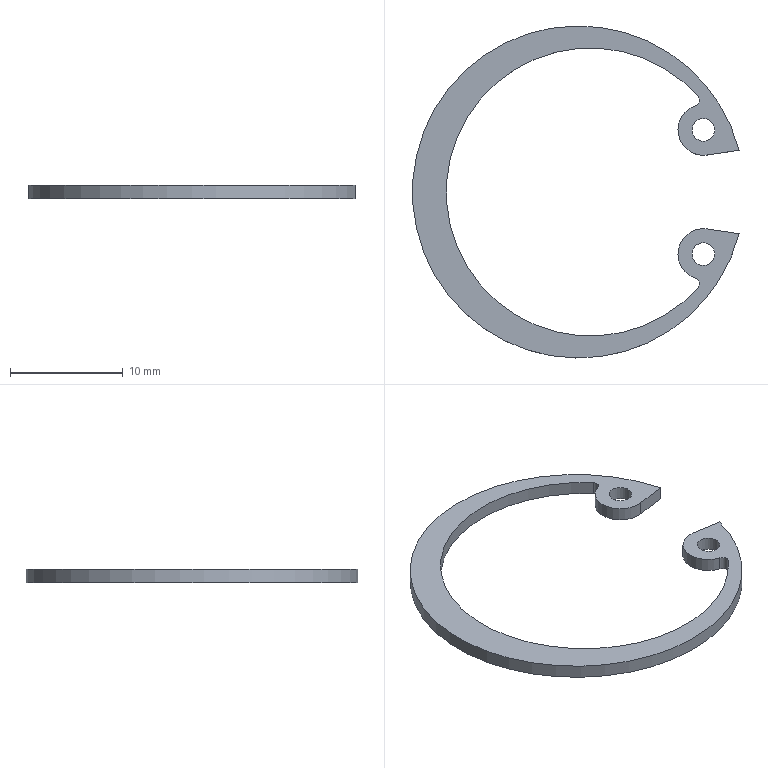Part | NX | features Retaining Ring C In-1_5003_005_BGRB6902ZZ-25 2 | 1 solid | 12 faces | box 28.927 x 29.4 x 1.2 mm | volume 220.032 mm3 | cylinder 8 | plane 4 | commonest cylinder face diameters 1 x2 2 x2 4.498 x2 25.5 x1 29.4 x1
STEP:
#1=CARTESIAN_POINT('',(169.581,-317.5,-237.85));
#2=VERTEX_POINT('',#1);
#3=CARTESIAN_POINT('',(169.581,-316.5,-237.85));
#4=DIRECTION('',(0.,0.,-1.));
#5=DIRECTION('',(0.,-1.,0.));
#6=AXIS2_PLACEMENT_3D('',#3,#4,#5);
#7=CIRCLE('',#6,1.);
#8=EDGE_CURVE('',#2,#2,#7,.T.);
#9=ORIENTED_EDGE('',*,*,#8,.F.);
#10=EDGE_LOOP('',(#9));
#11=FACE_BOUND('',#10,.T.);
#12=CARTESIAN_POINT('',(169.914,-318.724,-237.85));
#13=VERTEX_POINT('',#12);
#14=CARTESIAN_POINT('',(168.899,-314.357,-237.85));
#15=VERTEX_POINT('',#14);
#16=CARTESIAN_POINT('',(169.581,-316.5,-237.85));
#17=DIRECTION('',(0.,0.,-1.));
#18=DIRECTION('',(0.,-1.,0.));
#19=AXIS2_PLACEMENT_3D('',#16,#17,#18);
#20=CIRCLE('',#19,2.249);
#21=EDGE_CURVE('',#13,#15,#20,.T.);
#22=ORIENTED_EDGE('',*,*,#21,.T.);
#23=CARTESIAN_POINT('',(169.122,-313.549,-237.85));
#24=VERTEX_POINT('',#23);
#25=CARTESIAN_POINT('',(168.748,-313.881,-237.85));
#26=DIRECTION('',(0.,0.,1.));
#27=DIRECTION('',(0.,-1.,0.));
#28=AXIS2_PLACEMENT_3D('',#25,#26,#27);
#29=CIRCLE('',#28,0.5);
#30=EDGE_CURVE('',#15,#24,#29,.T.);
#31=ORIENTED_EDGE('',*,*,#30,.T.);
#32=CARTESIAN_POINT('',(169.122,-330.451,-237.85));
#33=VERTEX_POINT('',#32);
#34=CARTESIAN_POINT('',(159.575,-322.,-237.85));
#35=DIRECTION('',(0.,0.,1.));
#36=DIRECTION('',(0.,-1.,0.));
#37=AXIS2_PLACEMENT_3D('',#34,#35,#36);
#38=CIRCLE('',#37,12.75);
#39=EDGE_CURVE('',#24,#33,#38,.T.);
#40=ORIENTED_EDGE('',*,*,#39,.T.);
#41=CARTESIAN_POINT('',(168.899,-329.643,-237.85));
#42=VERTEX_POINT('',#41);
#43=CARTESIAN_POINT('',(168.748,-330.119,-237.85));
#44=DIRECTION('',(0.,0.,1.));
#45=DIRECTION('',(0.,1.,0.));
#46=AXIS2_PLACEMENT_3D('',#43,#44,#45);
#47=CIRCLE('',#46,0.5);
#48=EDGE_CURVE('',#33,#42,#47,.T.);
#49=ORIENTED_EDGE('',*,*,#48,.T.);
#50=CARTESIAN_POINT('',(169.914,-325.276,-237.85));
#51=VERTEX_POINT('',#50);
#52=CARTESIAN_POINT('',(169.581,-327.5,-237.85));
#53=DIRECTION('',(0.,0.,-1.));
#54=DIRECTION('',(0.,-1.,0.));
#55=AXIS2_PLACEMENT_3D('',#52,#53,#54);
#56=CIRCLE('',#55,2.249);
#57=EDGE_CURVE('',#42,#51,#56,.T.);
#58=ORIENTED_EDGE('',*,*,#57,.T.);
#59=CARTESIAN_POINT('',(172.752,-325.7,-237.85));
#60=VERTEX_POINT('',#59);
#61=CARTESIAN_POINT('',(169.914,-325.276,-237.85));
#62=DIRECTION('',(0.989,-0.1478,0.));
#63=VECTOR('',#62,1000.);
#64=LINE('',#61,#63);
#65=EDGE_CURVE('',#51,#60,#64,.T.);
#66=ORIENTED_EDGE('',*,*,#65,.T.);
#67=CARTESIAN_POINT('',(172.752,-318.3,-237.85));
#68=VERTEX_POINT('',#67);
#69=CARTESIAN_POINT('',(158.525,-322.,-237.85));
#70=DIRECTION('',(0.,0.,-1.));
#71=DIRECTION('',(0.,-1.,0.));
#72=AXIS2_PLACEMENT_3D('',#69,#70,#71);
#73=CIRCLE('',#72,14.7);
#74=EDGE_CURVE('',#60,#68,#73,.T.);
#75=ORIENTED_EDGE('',*,*,#74,.T.);
#76=CARTESIAN_POINT('',(169.914,-318.724,-237.85));
#77=DIRECTION('',(-0.989,-0.1478,0.));
#78=VECTOR('',#77,1000.);
#79=LINE('',#76,#78);
#80=EDGE_CURVE('',#68,#13,#79,.T.);
#81=ORIENTED_EDGE('',*,*,#80,.T.);
#82=EDGE_LOOP('',(#22,#31,#40,#49,#58,#66,#75,#81));
#83=FACE_BOUND('',#82,.T.);
#84=CARTESIAN_POINT('',(169.581,-328.5,-237.85));
#85=VERTEX_POINT('',#84);
#86=CARTESIAN_POINT('',(169.581,-327.5,-237.85));
#87=DIRECTION('',(0.,0.,-1.));
#88=DIRECTION('',(0.,-1.,0.));
#89=AXIS2_PLACEMENT_3D('',#86,#87,#88);
#90=CIRCLE('',#89,1.);
#91=EDGE_CURVE('',#85,#85,#90,.T.);
#92=ORIENTED_EDGE('',*,*,#91,.F.);
#93=EDGE_LOOP('',(#92));
#94=FACE_BOUND('',#93,.T.);
#95=CARTESIAN_POINT('',(169.581,-316.5,-237.85));
#96=DIRECTION('',(0.,0.,-1.));
#97=DIRECTION('',(0.,-1.,0.));
#98=AXIS2_PLACEMENT_3D('',#95,#96,#97);
#99=PLANE('',#98);
#100=ADVANCED_FACE('',(#11,#83,#94),#99,.T.);
#101=CARTESIAN_POINT('',(169.581,-317.5,-236.65));
#102=VERTEX_POINT('',#101);
#103=CARTESIAN_POINT('',(169.581,-316.5,-236.65));
#104=DIRECTION('',(0.,0.,-1.));
#105=DIRECTION('',(0.,-1.,0.));
#106=AXIS2_PLACEMENT_3D('',#103,#104,#105);
#107=CIRCLE('',#106,1.);
#108=EDGE_CURVE('',#102,#102,#107,.T.);
#109=ORIENTED_EDGE('',*,*,#108,.T.);
#110=EDGE_LOOP('',(#109));
#111=FACE_BOUND('',#110,.T.);
#112=CARTESIAN_POINT('',(169.914,-318.724,-236.65));
#113=VERTEX_POINT('',#112);
#114=CARTESIAN_POINT('',(168.899,-314.357,-236.65));
#115=VERTEX_POINT('',#114);
#116=CARTESIAN_POINT('',(169.581,-316.5,-236.65));
#117=DIRECTION('',(0.,0.,-1.));
#118=DIRECTION('',(0.,-1.,0.));
#119=AXIS2_PLACEMENT_3D('',#116,#117,#118);
#120=CIRCLE('',#119,2.249);
#121=EDGE_CURVE('',#113,#115,#120,.T.);
#122=ORIENTED_EDGE('',*,*,#121,.F.);
#123=CARTESIAN_POINT('',(172.752,-318.3,-236.65));
#124=VERTEX_POINT('',#123);
#125=CARTESIAN_POINT('',(169.914,-318.724,-236.65));
#126=DIRECTION('',(-0.989,-0.1478,0.));
#127=VECTOR('',#126,1000.);
#128=LINE('',#125,#127);
#129=EDGE_CURVE('',#124,#113,#128,.T.);
#130=ORIENTED_EDGE('',*,*,#129,.F.);
#131=CARTESIAN_POINT('',(172.752,-325.7,-236.65));
#132=VERTEX_POINT('',#131);
#133=CARTESIAN_POINT('',(158.525,-322.,-236.65));
#134=DIRECTION('',(0.,0.,-1.));
#135=DIRECTION('',(0.,-1.,0.));
#136=AXIS2_PLACEMENT_3D('',#133,#134,#135);
#137=CIRCLE('',#136,14.7);
#138=EDGE_CURVE('',#132,#124,#137,.T.);
#139=ORIENTED_EDGE('',*,*,#138,.F.);
#140=CARTESIAN_POINT('',(169.914,-325.276,-236.65));
#141=VERTEX_POINT('',#140);
#142=CARTESIAN_POINT('',(169.914,-325.276,-236.65));
#143=DIRECTION('',(0.989,-0.1478,0.));
#144=VECTOR('',#143,1000.);
#145=LINE('',#142,#144);
#146=EDGE_CURVE('',#141,#132,#145,.T.);
#147=ORIENTED_EDGE('',*,*,#146,.F.);
#148=CARTESIAN_POINT('',(168.899,-329.643,-236.65));
#149=VERTEX_POINT('',#148);
#150=CARTESIAN_POINT('',(169.581,-327.5,-236.65));
#151=DIRECTION('',(0.,0.,-1.));
#152=DIRECTION('',(0.,-1.,0.));
#153=AXIS2_PLACEMENT_3D('',#150,#151,#152);
#154=CIRCLE('',#153,2.249);
#155=EDGE_CURVE('',#149,#141,#154,.T.);
#156=ORIENTED_EDGE('',*,*,#155,.F.);
#157=CARTESIAN_POINT('',(169.122,-330.451,-236.65));
#158=VERTEX_POINT('',#157);
#159=CARTESIAN_POINT('',(168.748,-330.119,-236.65));
#160=DIRECTION('',(0.,0.,1.));
#161=DIRECTION('',(0.,1.,0.));
#162=AXIS2_PLACEMENT_3D('',#159,#160,#161);
#163=CIRCLE('',#162,0.5);
#164=EDGE_CURVE('',#158,#149,#163,.T.);
#165=ORIENTED_EDGE('',*,*,#164,.F.);
#166=CARTESIAN_POINT('',(169.122,-313.549,-236.65));
#167=VERTEX_POINT('',#166);
#168=CARTESIAN_POINT('',(159.575,-322.,-236.65));
#169=DIRECTION('',(0.,0.,1.));
#170=DIRECTION('',(0.,-1.,0.));
#171=AXIS2_PLACEMENT_3D('',#168,#169,#170);
#172=CIRCLE('',#171,12.75);
#173=EDGE_CURVE('',#167,#158,#172,.T.);
#174=ORIENTED_EDGE('',*,*,#173,.F.);
#175=CARTESIAN_POINT('',(168.748,-313.881,-236.65));
#176=DIRECTION('',(0.,0.,1.));
#177=DIRECTION('',(0.,-1.,0.));
#178=AXIS2_PLACEMENT_3D('',#175,#176,#177);
#179=CIRCLE('',#178,0.5);
#180=EDGE_CURVE('',#115,#167,#179,.T.);
#181=ORIENTED_EDGE('',*,*,#180,.F.);
#182=EDGE_LOOP('',(#122,#130,#139,#147,#156,#165,#174,#181));
#183=FACE_BOUND('',#182,.T.);
#184=CARTESIAN_POINT('',(169.581,-328.5,-236.65));
#185=VERTEX_POINT('',#184);
#186=CARTESIAN_POINT('',(169.581,-327.5,-236.65));
#187=DIRECTION('',(0.,0.,-1.));
#188=DIRECTION('',(0.,-1.,0.));
#189=AXIS2_PLACEMENT_3D('',#186,#187,#188);
#190=CIRCLE('',#189,1.);
#191=EDGE_CURVE('',#185,#185,#190,.T.);
#192=ORIENTED_EDGE('',*,*,#191,.T.);
#193=EDGE_LOOP('',(#192));
#194=FACE_BOUND('',#193,.T.);
#195=CARTESIAN_POINT('',(169.581,-316.5,-236.65));
#196=DIRECTION('',(0.,0.,-1.));
#197=DIRECTION('',(0.,-1.,0.));
#198=AXIS2_PLACEMENT_3D('',#195,#196,#197);
#199=PLANE('',#198);
#200=ADVANCED_FACE('',(#111,#183,#194),#199,.F.);
#201=ORIENTED_EDGE('',*,*,#121,.T.);
#202=CARTESIAN_POINT('',(168.899,-314.357,-237.85));
#203=DIRECTION('',(0.,0.,1.));
#204=VECTOR('',#203,1000.);
#205=LINE('',#202,#204);
#206=EDGE_CURVE('',#15,#115,#205,.T.);
#207=ORIENTED_EDGE('',*,*,#206,.F.);
#208=ORIENTED_EDGE('',*,*,#21,.F.);
#209=CARTESIAN_POINT('',(169.914,-318.724,-237.85));
#210=DIRECTION('',(0.,0.,1.));
#211=VECTOR('',#210,1000.);
#212=LINE('',#209,#211);
#213=EDGE_CURVE('',#13,#113,#212,.T.);
#214=ORIENTED_EDGE('',*,*,#213,.T.);
#215=EDGE_LOOP('',(#201,#207,#208,#214));
#216=FACE_BOUND('',#215,.T.);
#217=CARTESIAN_POINT('',(169.581,-316.5,-237.85));
#218=DIRECTION('',(0.,0.,1.));
#219=DIRECTION('',(0.,1.,0.));
#220=AXIS2_PLACEMENT_3D('',#217,#218,#219);
#221=CYLINDRICAL_SURFACE('',#220,2.249);
#222=ADVANCED_FACE('',(#216),#221,.T.);
#223=ORIENTED_EDGE('',*,*,#180,.T.);
#224=CARTESIAN_POINT('',(169.122,-313.549,-237.85));
#225=DIRECTION('',(0.,0.,1.));
#226=VECTOR('',#225,1000.);
#227=LINE('',#224,#226);
#228=EDGE_CURVE('',#24,#167,#227,.T.);
#229=ORIENTED_EDGE('',*,*,#228,.F.);
#230=ORIENTED_EDGE('',*,*,#30,.F.);
#231=ORIENTED_EDGE('',*,*,#206,.T.);
#232=EDGE_LOOP('',(#223,#229,#230,#231));
#233=FACE_BOUND('',#232,.T.);
#234=CARTESIAN_POINT('',(168.748,-313.881,-237.85));
#235=DIRECTION('',(0.,0.,1.));
#236=DIRECTION('',(0.,1.,0.));
#237=AXIS2_PLACEMENT_3D('',#234,#235,#236);
#238=CYLINDRICAL_SURFACE('',#237,0.5);
#239=ADVANCED_FACE('',(#233),#238,.F.);
#240=ORIENTED_EDGE('',*,*,#173,.T.);
#241=CARTESIAN_POINT('',(169.122,-330.451,-237.85));
#242=DIRECTION('',(0.,0.,1.));
#243=VECTOR('',#242,1000.);
#244=LINE('',#241,#243);
#245=EDGE_CURVE('',#33,#158,#244,.T.);
#246=ORIENTED_EDGE('',*,*,#245,.F.);
#247=ORIENTED_EDGE('',*,*,#39,.F.);
#248=ORIENTED_EDGE('',*,*,#228,.T.);
#249=EDGE_LOOP('',(#240,#246,#247,#248));
#250=FACE_BOUND('',#249,.T.);
#251=CARTESIAN_POINT('',(159.575,-322.,-237.85));
#252=DIRECTION('',(0.,0.,1.));
#253=DIRECTION('',(0.,1.,0.));
#254=AXIS2_PLACEMENT_3D('',#251,#252,#253);
#255=CYLINDRICAL_SURFACE('',#254,12.75);
#256=ADVANCED_FACE('',(#250),#255,.F.);
#257=ORIENTED_EDGE('',*,*,#164,.T.);
#258=CARTESIAN_POINT('',(168.899,-329.643,-237.85));
#259=DIRECTION('',(0.,0.,1.));
#260=VECTOR('',#259,1000.);
#261=LINE('',#258,#260);
#262=EDGE_CURVE('',#42,#149,#261,.T.);
#263=ORIENTED_EDGE('',*,*,#262,.F.);
#264=ORIENTED_EDGE('',*,*,#48,.F.);
#265=ORIENTED_EDGE('',*,*,#245,.T.);
#266=EDGE_LOOP('',(#257,#263,#264,#265));
#267=FACE_BOUND('',#266,.T.);
#268=CARTESIAN_POINT('',(168.748,-330.119,-237.85));
#269=DIRECTION('',(0.,0.,1.));
#270=DIRECTION('',(0.,1.,0.));
#271=AXIS2_PLACEMENT_3D('',#268,#269,#270);
#272=CYLINDRICAL_SURFACE('',#271,0.5);
#273=ADVANCED_FACE('',(#267),#272,.F.);
#274=ORIENTED_EDGE('',*,*,#155,.T.);
#275=CARTESIAN_POINT('',(169.914,-325.276,-237.85));
#276=DIRECTION('',(0.,0.,1.));
#277=VECTOR('',#276,1000.);
#278=LINE('',#275,#277);
#279=EDGE_CURVE('',#51,#141,#278,.T.);
#280=ORIENTED_EDGE('',*,*,#279,.F.);
#281=ORIENTED_EDGE('',*,*,#57,.F.);
#282=ORIENTED_EDGE('',*,*,#262,.T.);
#283=EDGE_LOOP('',(#274,#280,#281,#282));
#284=FACE_BOUND('',#283,.T.);
#285=CARTESIAN_POINT('',(169.581,-327.5,-237.85));
#286=DIRECTION('',(0.,0.,1.));
#287=DIRECTION('',(0.,1.,0.));
#288=AXIS2_PLACEMENT_3D('',#285,#286,#287);
#289=CYLINDRICAL_SURFACE('',#288,2.249);
#290=ADVANCED_FACE('',(#284),#289,.T.);
#291=ORIENTED_EDGE('',*,*,#146,.T.);
#292=CARTESIAN_POINT('',(172.752,-325.7,-237.85));
#293=DIRECTION('',(0.,0.,1.));
#294=VECTOR('',#293,1000.);
#295=LINE('',#292,#294);
#296=EDGE_CURVE('',#60,#132,#295,.T.);
#297=ORIENTED_EDGE('',*,*,#296,.F.);
#298=ORIENTED_EDGE('',*,*,#65,.F.);
#299=ORIENTED_EDGE('',*,*,#279,.T.);
#300=EDGE_LOOP('',(#291,#297,#298,#299));
#301=FACE_BOUND('',#300,.T.);
#302=CARTESIAN_POINT('',(169.914,-325.276,-237.85));
#303=DIRECTION('',(-0.1478,-0.989,0.));
#304=DIRECTION('',(-0.989,0.1478,0.));
#305=AXIS2_PLACEMENT_3D('',#302,#303,#304);
#306=PLANE('',#305);
#307=ADVANCED_FACE('',(#301),#306,.F.);
#308=ORIENTED_EDGE('',*,*,#138,.T.);
#309=CARTESIAN_POINT('',(172.752,-318.3,-237.85));
#310=DIRECTION('',(0.,0.,1.));
#311=VECTOR('',#310,1000.);
#312=LINE('',#309,#311);
#313=EDGE_CURVE('',#68,#124,#312,.T.);
#314=ORIENTED_EDGE('',*,*,#313,.F.);
#315=ORIENTED_EDGE('',*,*,#74,.F.);
#316=ORIENTED_EDGE('',*,*,#296,.T.);
#317=EDGE_LOOP('',(#308,#314,#315,#316));
#318=FACE_BOUND('',#317,.T.);
#319=CARTESIAN_POINT('',(158.525,-322.,-237.85));
#320=DIRECTION('',(0.,0.,1.));
#321=DIRECTION('',(0.,1.,0.));
#322=AXIS2_PLACEMENT_3D('',#319,#320,#321);
#323=CYLINDRICAL_SURFACE('',#322,14.7);
#324=ADVANCED_FACE('',(#318),#323,.T.);
#325=ORIENTED_EDGE('',*,*,#129,.T.);
#326=ORIENTED_EDGE('',*,*,#213,.F.);
#327=ORIENTED_EDGE('',*,*,#80,.F.);
#328=ORIENTED_EDGE('',*,*,#313,.T.);
#329=EDGE_LOOP('',(#325,#326,#327,#328));
#330=FACE_BOUND('',#329,.T.);
#331=CARTESIAN_POINT('',(169.914,-318.724,-237.85));
#332=DIRECTION('',(-0.1478,0.989,0.));
#333=DIRECTION('',(0.989,0.1478,0.));
#334=AXIS2_PLACEMENT_3D('',#331,#332,#333);
#335=PLANE('',#334);
#336=ADVANCED_FACE('',(#330),#335,.F.);
#337=ORIENTED_EDGE('',*,*,#8,.T.);
#338=EDGE_LOOP('',(#337));
#339=FACE_BOUND('',#338,.T.);
#340=ORIENTED_EDGE('',*,*,#108,.F.);
#341=EDGE_LOOP('',(#340));
#342=FACE_BOUND('',#341,.T.);
#343=CARTESIAN_POINT('',(169.581,-316.5,-237.85));
#344=DIRECTION('',(0.,0.,1.));
#345=DIRECTION('',(0.,1.,0.));
#346=AXIS2_PLACEMENT_3D('',#343,#344,#345);
#347=CYLINDRICAL_SURFACE('',#346,1.);
#348=ADVANCED_FACE('',(#339,#342),#347,.F.);
#349=ORIENTED_EDGE('',*,*,#91,.T.);
#350=EDGE_LOOP('',(#349));
#351=FACE_BOUND('',#350,.T.);
#352=ORIENTED_EDGE('',*,*,#191,.F.);
#353=EDGE_LOOP('',(#352));
#354=FACE_BOUND('',#353,.T.);
#355=CARTESIAN_POINT('',(169.581,-327.5,-237.85));
#356=DIRECTION('',(0.,0.,1.));
#357=DIRECTION('',(0.,1.,0.));
#358=AXIS2_PLACEMENT_3D('',#355,#356,#357);
#359=CYLINDRICAL_SURFACE('',#358,1.);
#360=ADVANCED_FACE('',(#351,#354),#359,.F.);
#361=CLOSED_SHELL('',(#100,#200,#222,#239,#256,#273,#290,#307,#324,#336,#348,#360));
#362=MANIFOLD_SOLID_BREP('',#361);
#363=(LENGTH_UNIT()NAMED_UNIT(*)SI_UNIT(.MILLI.,.METRE.));
#364=UNCERTAINTY_MEASURE_WITH_UNIT(LENGTH_MEASURE(0.00001),#363,'','');
#365=(NAMED_UNIT(*)PLANE_ANGLE_UNIT()SI_UNIT($,.RADIAN.));
#366=(NAMED_UNIT(*)SI_UNIT($,.STERADIAN.)SOLID_ANGLE_UNIT());
#367=(GEOMETRIC_REPRESENTATION_CONTEXT(3)GLOBAL_UNCERTAINTY_ASSIGNED_CONTEXT((#364))GLOBAL_UNIT_ASSIGNED_CONTEXT((#363,#365,#366))REPRESENTATION_CONTEXT('',''));
#368=ADVANCED_BREP_SHAPE_REPRESENTATION('',(#362),#367);